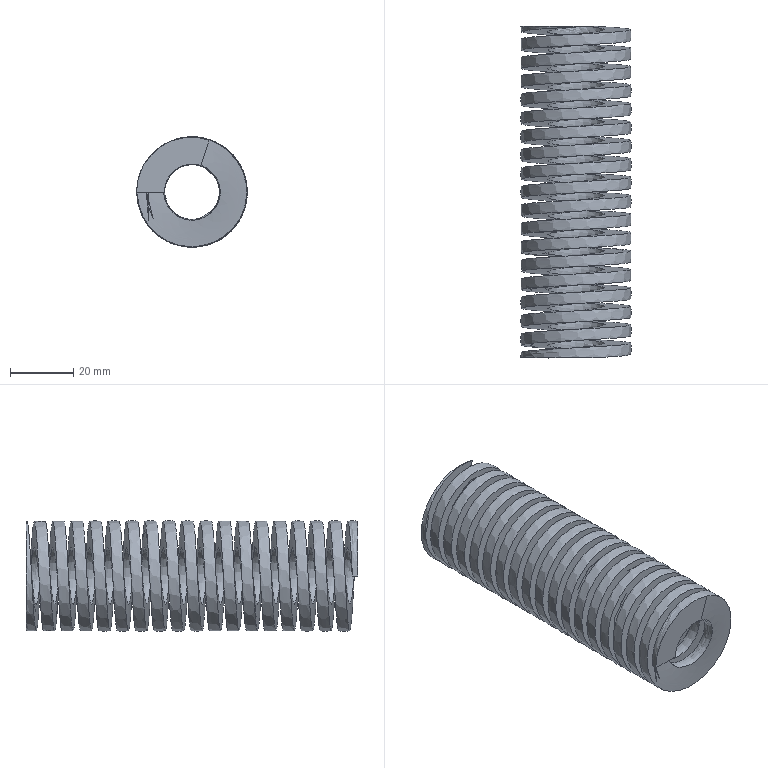Part | Creo | 1 solid | 7 faces | box 35 x 105.001 x 35 mm | volume 44219 mm3 | spline 4 | plane 3